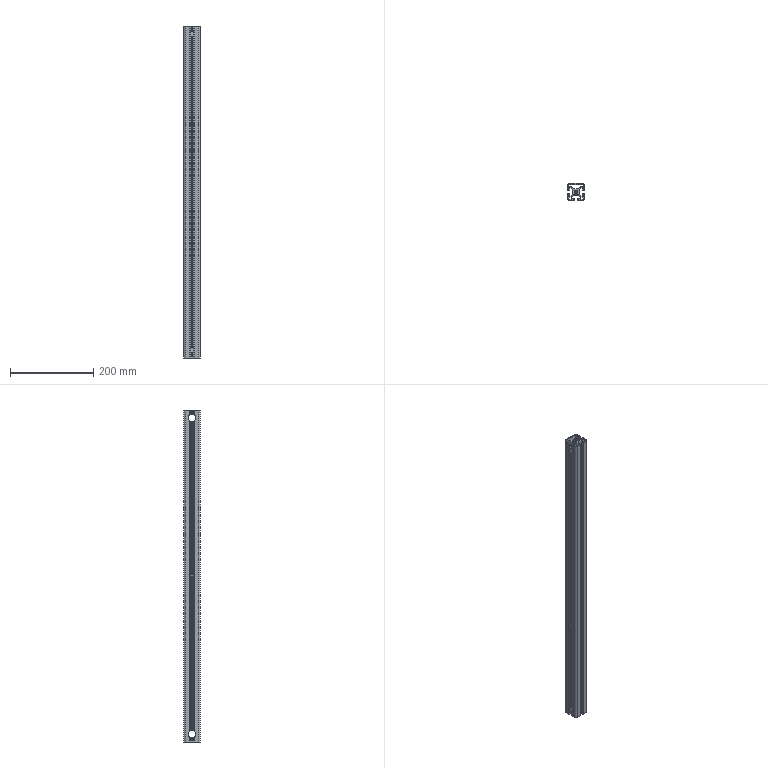Part | SolidWorks | features BaseBody 1, HoleWzd 1, MoveFace 1 | 1 solid | 242 faces | box 40 x 40 x 798 mm | volume 464090 mm3 | plane 187 | cylinder 55 | commonest cylinder face diameters 6.8 x15 2 x14 19 x12 1 x6 5 x4 9 x4